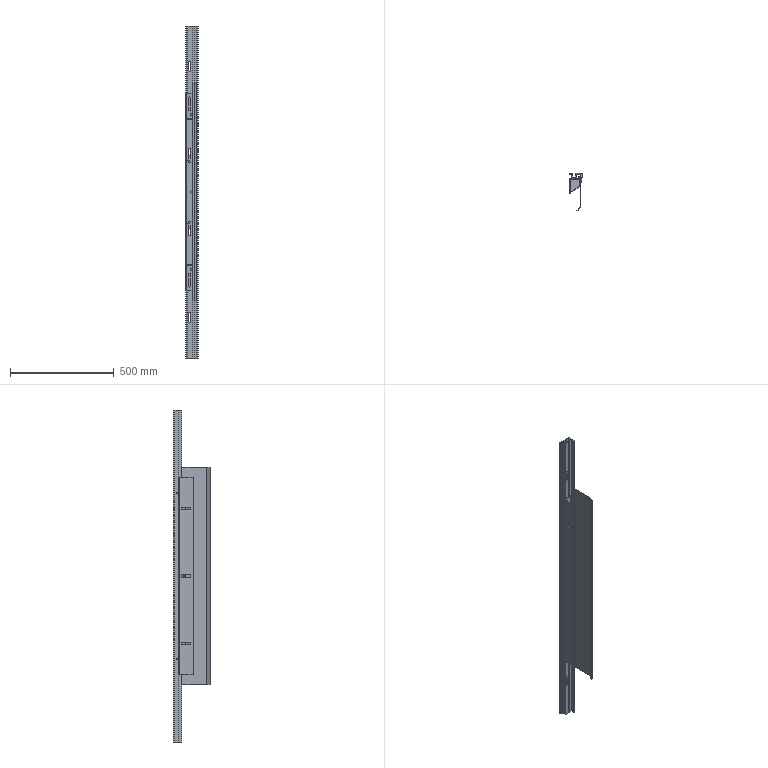Part | SolidWorks | 7 solids | 218 faces | box 60 x 178.321 x 1600 mm | volume 1702820 mm3 | plane 148 | cylinder 70 | commonest cylinder face diameters 10 x27 7 x15 2 x11 14 x8 3 x4 1 x2